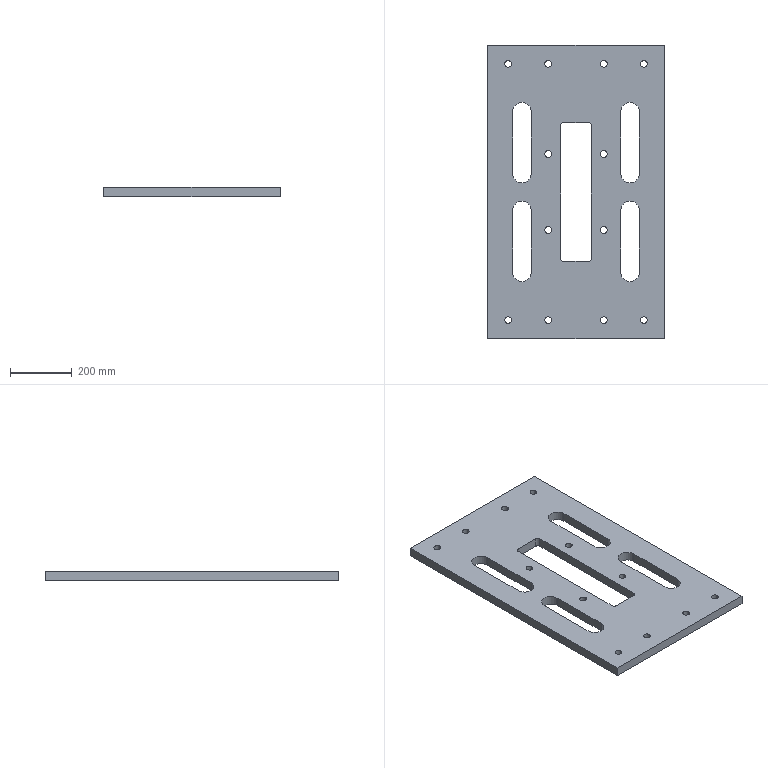Part | SolidWorks | features Extrusion 1 | 1 solid | 54 faces | box 570 x 950 x 30 mm | volume 12981435 mm3 | cylinder 36 | plane 18 | commonest cylinder face diameters 22 x24 60 x8 20 x4